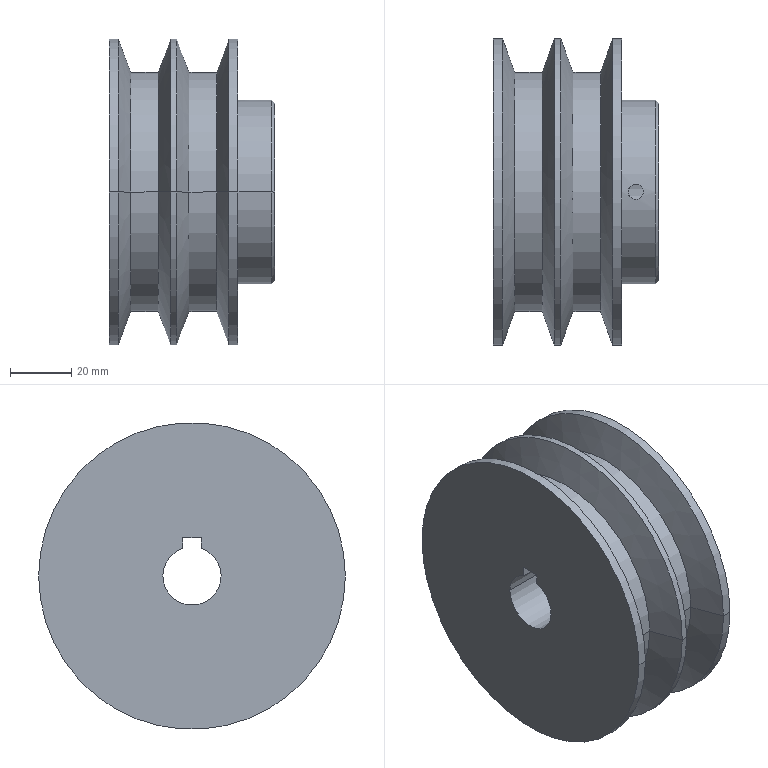Part | SolidWorks | features ICE 2, Chamfer 1, HoleWzd 1, Revolution 1 | 1 solid | 33 faces | box 54 x 100 x 100 mm | volume 266067 mm3 | cylinder 17 | cone 10 | plane 6 | commonest cylinder face diameters 100 x6 78 x4 19 x3 5 x2 60 x2
STEP:
#1=CARTESIAN_POINT('',(54.,29.,0.));
#2=VERTEX_POINT('',#1);
#3=CARTESIAN_POINT('',(54.,-29.,0.));
#4=VERTEX_POINT('',#3);
#5=CARTESIAN_POINT('',(54.,0.,0.));
#6=DIRECTION('',(1.,0.,0.));
#7=DIRECTION('',(0.,1.,0.));
#8=AXIS2_PLACEMENT_3D('',#5,#6,#7);
#9=CIRCLE('',#8,29.);
#10=EDGE_CURVE('',#2,#4,#9,.T.);
#11=ORIENTED_EDGE('',*,*,#10,.F.);
#12=CARTESIAN_POINT('',(53.,30.,0.));
#13=VERTEX_POINT('',#12);
#14=CARTESIAN_POINT('',(54.,29.,0.));
#15=DIRECTION('',(-0.7071,0.7071,0.));
#16=VECTOR('',#15,1000.);
#17=LINE('',#14,#16);
#18=EDGE_CURVE('',#2,#13,#17,.T.);
#19=ORIENTED_EDGE('',*,*,#18,.T.);
#20=CARTESIAN_POINT('',(53.,-30.,0.));
#21=VERTEX_POINT('',#20);
#22=CARTESIAN_POINT('',(53.,0.,0.));
#23=DIRECTION('',(-1.,0.,0.));
#24=DIRECTION('',(0.,1.,0.));
#25=AXIS2_PLACEMENT_3D('',#22,#23,#24);
#26=CIRCLE('',#25,30.);
#27=EDGE_CURVE('',#21,#13,#26,.T.);
#28=ORIENTED_EDGE('',*,*,#27,.F.);
#29=CARTESIAN_POINT('',(54.,-29.,0.));
#30=DIRECTION('',(-0.7071,-0.7071,0.));
#31=VECTOR('',#30,1000.);
#32=LINE('',#29,#31);
#33=EDGE_CURVE('',#4,#21,#32,.T.);
#34=ORIENTED_EDGE('',*,*,#33,.F.);
#35=EDGE_LOOP('',(#11,#19,#28,#34));
#36=FACE_OUTER_BOUND('',#35,.T.);
#37=CARTESIAN_POINT('',(54.,0.,0.));
#38=DIRECTION('',(-1.,0.,0.));
#39=DIRECTION('',(0.,-1.,0.));
#40=AXIS2_PLACEMENT_3D('',#37,#38,#39);
#41=CONICAL_SURFACE('',#40,29.,0.7854);
#42=ADVANCED_FACE('',(#36),#41,.T.);
#43=CARTESIAN_POINT('',(44.,0.,30.));
#44=VERTEX_POINT('',#43);
#45=CARTESIAN_POINT('',(49.,0.,30.));
#46=VERTEX_POINT('',#45);
#47=CARTESIAN_POINT('',(44.,0.,30.));
#48=CARTESIAN_POINT('',(44.,-0.1653,30.));
#49=CARTESIAN_POINT('',(44.016,-0.3277,29.999));
#50=CARTESIAN_POINT('',(44.08,-0.6474,29.993));
#51=CARTESIAN_POINT('',(44.128,-0.8062,29.99));
#52=CARTESIAN_POINT('',(44.253,-1.109,29.98));
#53=CARTESIAN_POINT('',(44.33,-1.253,29.974));
#54=CARTESIAN_POINT('',(44.512,-1.524,29.962));
#55=CARTESIAN_POINT('',(44.617,-1.653,29.955));
#56=CARTESIAN_POINT('',(44.848,-1.883,29.941));
#57=CARTESIAN_POINT('',(44.974,-1.987,29.934));
#58=CARTESIAN_POINT('',(45.247,-2.17,29.922));
#59=CARTESIAN_POINT('',(45.392,-2.247,29.916));
#60=CARTESIAN_POINT('',(45.693,-2.372,29.906));
#61=CARTESIAN_POINT('',(45.851,-2.42,29.902));
#62=CARTESIAN_POINT('',(46.174,-2.484,29.897));
#63=CARTESIAN_POINT('',(46.336,-2.5,29.896));
#64=CARTESIAN_POINT('',(46.662,-2.5,29.896));
#65=CARTESIAN_POINT('',(46.828,-2.484,29.897));
#66=CARTESIAN_POINT('',(47.149,-2.42,29.902));
#67=CARTESIAN_POINT('',(47.305,-2.373,29.906));
#68=CARTESIAN_POINT('',(47.607,-2.247,29.916));
#69=CARTESIAN_POINT('',(47.754,-2.169,29.922));
#70=CARTESIAN_POINT('',(48.024,-1.988,29.934));
#71=CARTESIAN_POINT('',(48.151,-1.885,29.941));
#72=CARTESIAN_POINT('',(48.384,-1.651,29.955));
#73=CARTESIAN_POINT('',(48.488,-1.525,29.962));
#74=CARTESIAN_POINT('',(48.669,-1.254,29.974));
#75=CARTESIAN_POINT('',(48.747,-1.108,29.98));
#76=CARTESIAN_POINT('',(48.872,-0.8053,29.99));
#77=CARTESIAN_POINT('',(48.92,-0.6495,29.993));
#78=CARTESIAN_POINT('',(48.984,-0.329,29.999));
#79=CARTESIAN_POINT('',(49.,-0.1632,30.));
#80=CARTESIAN_POINT('',(49.,0.,30.));
#81=B_SPLINE_CURVE_WITH_KNOTS('',3,(#47,#48,#49,#50,#51,#52,#53,#54,#55,#56,#57,#58,#59,#60,#61,#62,#63,#64,#65,#66,#67,#68,#69,#70,#71,#72,#73,#74,#75,#76,#77,#78,#79,#80),.UNSPECIFIED.,.F.,.F.,(4,2,2,2,2,2,2,2,2,2,2,2,2,2,2,2,4),(0.,0.0004887,0.0009774,0.001466,0.001955,0.002444,0.002932,0.003421,0.00391,0.004398,0.004887,0.005376,0.005865,0.006353,0.006842,0.007331,0.00782),.UNSPECIFIED.);
#82=EDGE_CURVE('',#44,#46,#81,.T.);
#83=ORIENTED_EDGE('',*,*,#82,.T.);
#84=CARTESIAN_POINT('',(49.,0.,12.5));
#85=VERTEX_POINT('',#84);
#86=CARTESIAN_POINT('',(49.,0.,0.));
#87=DIRECTION('',(0.,0.,-1.));
#88=VECTOR('',#87,1000.);
#89=LINE('',#86,#88);
#90=EDGE_CURVE('',#46,#85,#89,.T.);
#91=ORIENTED_EDGE('',*,*,#90,.T.);
#92=CARTESIAN_POINT('',(44.,0.,12.5));
#93=VERTEX_POINT('',#92);
#94=CARTESIAN_POINT('',(46.5,0.,12.5));
#95=DIRECTION('',(0.,0.,-1.));
#96=DIRECTION('',(1.,0.,0.));
#97=AXIS2_PLACEMENT_3D('',#94,#95,#96);
#98=CIRCLE('',#97,2.5);
#99=EDGE_CURVE('',#85,#93,#98,.T.);
#100=ORIENTED_EDGE('',*,*,#99,.T.);
#101=CARTESIAN_POINT('',(44.,0.,0.));
#102=DIRECTION('',(0.,0.,-1.));
#103=VECTOR('',#102,1000.);
#104=LINE('',#101,#103);
#105=EDGE_CURVE('',#44,#93,#104,.T.);
#106=ORIENTED_EDGE('',*,*,#105,.F.);
#107=EDGE_LOOP('',(#83,#91,#100,#106));
#108=FACE_OUTER_BOUND('',#107,.T.);
#109=CARTESIAN_POINT('',(46.5,0.,0.));
#110=DIRECTION('',(0.,0.,-1.));
#111=DIRECTION('',(-1.,0.,0.));
#112=AXIS2_PLACEMENT_3D('',#109,#110,#111);
#113=CYLINDRICAL_SURFACE('',#112,2.5);
#114=ADVANCED_FACE('',(#108),#113,.F.);
#115=CARTESIAN_POINT('',(0.,9.5,0.));
#116=VERTEX_POINT('',#115);
#117=CARTESIAN_POINT('',(0.,-9.5,0.));
#118=VERTEX_POINT('',#117);
#119=CARTESIAN_POINT('',(0.,0.,0.));
#120=DIRECTION('',(-1.,0.,0.));
#121=DIRECTION('',(0.,-1.,0.));
#122=AXIS2_PLACEMENT_3D('',#119,#120,#121);
#123=CIRCLE('',#122,9.5);
#124=EDGE_CURVE('',#116,#118,#123,.T.);
#125=ORIENTED_EDGE('',*,*,#124,.T.);
#126=CARTESIAN_POINT('',(54.,-9.5,0.));
#127=VERTEX_POINT('',#126);
#128=CARTESIAN_POINT('',(-16.,-9.5,0.));
#129=DIRECTION('',(1.,0.,0.));
#130=VECTOR('',#129,1000.);
#131=LINE('',#128,#130);
#132=EDGE_CURVE('',#118,#127,#131,.T.);
#133=ORIENTED_EDGE('',*,*,#132,.T.);
#134=CARTESIAN_POINT('',(54.,9.5,0.));
#135=VERTEX_POINT('',#134);
#136=CARTESIAN_POINT('',(54.,0.,0.));
#137=DIRECTION('',(1.,0.,0.));
#138=DIRECTION('',(0.,1.,0.));
#139=AXIS2_PLACEMENT_3D('',#136,#137,#138);
#140=CIRCLE('',#139,9.5);
#141=EDGE_CURVE('',#127,#135,#140,.T.);
#142=ORIENTED_EDGE('',*,*,#141,.T.);
#143=CARTESIAN_POINT('',(-16.,9.5,0.));
#144=DIRECTION('',(1.,0.,0.));
#145=VECTOR('',#144,1000.);
#146=LINE('',#143,#145);
#147=EDGE_CURVE('',#116,#135,#146,.T.);
#148=ORIENTED_EDGE('',*,*,#147,.F.);
#149=EDGE_LOOP('',(#125,#133,#142,#148));
#150=FACE_OUTER_BOUND('',#149,.T.);
#151=CARTESIAN_POINT('',(-16.,0.,0.));
#152=DIRECTION('',(1.,0.,0.));
#153=DIRECTION('',(0.,1.,0.));
#154=AXIS2_PLACEMENT_3D('',#151,#152,#153);
#155=CYLINDRICAL_SURFACE('',#154,9.5);
#156=ADVANCED_FACE('',(#150),#155,.F.);
#157=CARTESIAN_POINT('',(0.,3.,9.014));
#158=VERTEX_POINT('',#157);
#159=CARTESIAN_POINT('',(0.,0.,0.));
#160=DIRECTION('',(-1.,0.,0.));
#161=DIRECTION('',(0.,-1.,0.));
#162=AXIS2_PLACEMENT_3D('',#159,#160,#161);
#163=CIRCLE('',#162,9.5);
#164=EDGE_CURVE('',#158,#116,#163,.T.);
#165=ORIENTED_EDGE('',*,*,#164,.T.);
#166=ORIENTED_EDGE('',*,*,#147,.T.);
#167=CARTESIAN_POINT('',(54.,3.,9.014));
#168=VERTEX_POINT('',#167);
#169=CARTESIAN_POINT('',(54.,0.,0.));
#170=DIRECTION('',(1.,0.,0.));
#171=DIRECTION('',(0.,1.,0.));
#172=AXIS2_PLACEMENT_3D('',#169,#170,#171);
#173=CIRCLE('',#172,9.5);
#174=EDGE_CURVE('',#135,#168,#173,.T.);
#175=ORIENTED_EDGE('',*,*,#174,.T.);
#176=CARTESIAN_POINT('',(-16.,3.,9.014));
#177=DIRECTION('',(-1.,0.,0.));
#178=VECTOR('',#177,1000.);
#179=LINE('',#176,#178);
#180=EDGE_CURVE('',#168,#158,#179,.T.);
#181=ORIENTED_EDGE('',*,*,#180,.T.);
#182=EDGE_LOOP('',(#165,#166,#175,#181));
#183=FACE_OUTER_BOUND('',#182,.T.);
#184=CARTESIAN_POINT('',(-16.,0.,0.));
#185=DIRECTION('',(1.,0.,0.));
#186=DIRECTION('',(0.,1.,0.));
#187=AXIS2_PLACEMENT_3D('',#184,#185,#186);
#188=CYLINDRICAL_SURFACE('',#187,9.5);
#189=ADVANCED_FACE('',(#183),#188,.F.);
#190=ORIENTED_EDGE('',*,*,#82,.F.);
#191=CARTESIAN_POINT('',(49.,0.,30.));
#192=CARTESIAN_POINT('',(49.,0.1632,30.));
#193=CARTESIAN_POINT('',(48.984,0.3254,29.999));
#194=CARTESIAN_POINT('',(48.92,0.6478,29.993));
#195=CARTESIAN_POINT('',(48.872,0.8057,29.99));
#196=CARTESIAN_POINT('',(48.748,1.107,29.98));
#197=CARTESIAN_POINT('',(48.67,1.252,29.974));
#198=CARTESIAN_POINT('',(48.488,1.525,29.962));
#199=CARTESIAN_POINT('',(48.384,1.651,29.955));
#200=CARTESIAN_POINT('',(48.154,1.882,29.941));
#201=CARTESIAN_POINT('',(48.025,1.987,29.934));
#202=CARTESIAN_POINT('',(47.754,2.169,29.922));
#203=CARTESIAN_POINT('',(47.61,2.246,29.916));
#204=CARTESIAN_POINT('',(47.308,2.372,29.906));
#205=CARTESIAN_POINT('',(47.149,2.42,29.902));
#206=CARTESIAN_POINT('',(46.829,2.484,29.897));
#207=CARTESIAN_POINT('',(46.667,2.5,29.896));
#208=CARTESIAN_POINT('',(46.337,2.5,29.896));
#209=CARTESIAN_POINT('',(46.174,2.484,29.897));
#210=CARTESIAN_POINT('',(45.854,2.421,29.902));
#211=CARTESIAN_POINT('',(45.696,2.373,29.906));
#212=CARTESIAN_POINT('',(45.393,2.247,29.916));
#213=CARTESIAN_POINT('',(45.249,2.171,29.921));
#214=CARTESIAN_POINT('',(44.978,1.99,29.934));
#215=CARTESIAN_POINT('',(44.849,1.884,29.941));
#216=CARTESIAN_POINT('',(44.618,1.654,29.955));
#217=CARTESIAN_POINT('',(44.515,1.528,29.961));
#218=CARTESIAN_POINT('',(44.332,1.255,29.974));
#219=CARTESIAN_POINT('',(44.254,1.11,29.98));
#220=CARTESIAN_POINT('',(44.066,0.6587,29.994));
#221=CARTESIAN_POINT('',(44.,0.3304,30.));
#222=CARTESIAN_POINT('',(44.,0.,30.));
#223=B_SPLINE_CURVE_WITH_KNOTS('',3,(#191,#192,#193,#194,#195,#196,#197,#198,#199,#200,#201,#202,#203,#204,#205,#206,#207,#208,#209,#210,#211,#212,#213,#214,#215,#216,#217,#218,#219,#220,#221,#222),.UNSPECIFIED.,.F.,.F.,(4,2,2,2,2,2,2,2,2,2,2,2,2,2,2,4),(0.00782,0.008308,0.008797,0.009285,0.009774,0.01026,0.01075,0.01124,0.01173,0.01222,0.01271,0.01319,0.01368,0.01417,0.01466,0.01564),.UNSPECIFIED.);
#224=EDGE_CURVE('',#46,#44,#223,.T.);
#225=ORIENTED_EDGE('',*,*,#224,.F.);
#226=EDGE_LOOP('',(#190,#225));
#227=FACE_BOUND('',#226,.T.);
#228=CARTESIAN_POINT('',(42.,30.,0.));
#229=VERTEX_POINT('',#228);
#230=CARTESIAN_POINT('',(42.,-30.,0.));
#231=VERTEX_POINT('',#230);
#232=CARTESIAN_POINT('',(42.,0.,0.));
#233=DIRECTION('',(1.,0.,0.));
#234=DIRECTION('',(0.,1.,0.));
#235=AXIS2_PLACEMENT_3D('',#232,#233,#234);
#236=CIRCLE('',#235,30.);
#237=EDGE_CURVE('',#229,#231,#236,.T.);
#238=ORIENTED_EDGE('',*,*,#237,.T.);
#239=CARTESIAN_POINT('',(54.,-30.,0.));
#240=DIRECTION('',(1.,0.,0.));
#241=VECTOR('',#240,1000.);
#242=LINE('',#239,#241);
#243=EDGE_CURVE('',#231,#21,#242,.T.);
#244=ORIENTED_EDGE('',*,*,#243,.T.);
#245=ORIENTED_EDGE('',*,*,#27,.T.);
#246=CARTESIAN_POINT('',(54.,30.,0.));
#247=DIRECTION('',(1.,0.,0.));
#248=VECTOR('',#247,1000.);
#249=LINE('',#246,#248);
#250=EDGE_CURVE('',#229,#13,#249,.T.);
#251=ORIENTED_EDGE('',*,*,#250,.F.);
#252=EDGE_LOOP('',(#238,#244,#245,#251));
#253=FACE_OUTER_BOUND('',#252,.T.);
#254=CARTESIAN_POINT('',(54.,0.,0.));
#255=DIRECTION('',(1.,0.,0.));
#256=DIRECTION('',(0.,1.,0.));
#257=AXIS2_PLACEMENT_3D('',#254,#255,#256);
#258=CYLINDRICAL_SURFACE('',#257,30.);
#259=ADVANCED_FACE('',(#227,#253),#258,.T.);
#260=CARTESIAN_POINT('',(39.,50.,0.));
#261=VERTEX_POINT('',#260);
#262=CARTESIAN_POINT('',(39.,-50.,0.));
#263=VERTEX_POINT('',#262);
#264=CARTESIAN_POINT('',(39.,0.,0.));
#265=DIRECTION('',(1.,0.,0.));
#266=DIRECTION('',(0.,1.,0.));
#267=AXIS2_PLACEMENT_3D('',#264,#265,#266);
#268=CIRCLE('',#267,50.);
#269=EDGE_CURVE('',#261,#263,#268,.T.);
#270=ORIENTED_EDGE('',*,*,#269,.T.);
#271=CARTESIAN_POINT('',(42.,-50.,0.));
#272=VERTEX_POINT('',#271);
#273=CARTESIAN_POINT('',(54.,-50.,0.));
#274=DIRECTION('',(1.,0.,0.));
#275=VECTOR('',#274,1000.);
#276=LINE('',#273,#275);
#277=EDGE_CURVE('',#263,#272,#276,.T.);
#278=ORIENTED_EDGE('',*,*,#277,.T.);
#279=CARTESIAN_POINT('',(42.,50.,0.));
#280=VERTEX_POINT('',#279);
#281=CARTESIAN_POINT('',(42.,0.,0.));
#282=DIRECTION('',(1.,0.,0.));
#283=DIRECTION('',(0.,1.,0.));
#284=AXIS2_PLACEMENT_3D('',#281,#282,#283);
#285=CIRCLE('',#284,50.);
#286=EDGE_CURVE('',#280,#272,#285,.T.);
#287=ORIENTED_EDGE('',*,*,#286,.F.);
#288=CARTESIAN_POINT('',(54.,50.,0.));
#289=DIRECTION('',(1.,0.,0.));
#290=VECTOR('',#289,1000.);
#291=LINE('',#288,#290);
#292=EDGE_CURVE('',#261,#280,#291,.T.);
#293=ORIENTED_EDGE('',*,*,#292,.F.);
#294=EDGE_LOOP('',(#270,#278,#287,#293));
#295=FACE_OUTER_BOUND('',#294,.T.);
#296=CARTESIAN_POINT('',(54.,0.,0.));
#297=DIRECTION('',(1.,0.,0.));
#298=DIRECTION('',(0.,1.,0.));
#299=AXIS2_PLACEMENT_3D('',#296,#297,#298);
#300=CYLINDRICAL_SURFACE('',#299,50.);
#301=ADVANCED_FACE('',(#295),#300,.T.);
#302=CARTESIAN_POINT('',(34.996,39.,0.));
#303=VERTEX_POINT('',#302);
#304=CARTESIAN_POINT('',(34.996,-39.,0.));
#305=VERTEX_POINT('',#304);
#306=CARTESIAN_POINT('',(34.996,0.,0.));
#307=DIRECTION('',(1.,0.,0.));
#308=DIRECTION('',(0.,1.,0.));
#309=AXIS2_PLACEMENT_3D('',#306,#307,#308);
#310=CIRCLE('',#309,39.);
#311=EDGE_CURVE('',#303,#305,#310,.T.);
#312=ORIENTED_EDGE('',*,*,#311,.T.);
#313=CARTESIAN_POINT('',(39.,-50.,0.));
#314=DIRECTION('',(0.342,-0.9397,0.));
#315=VECTOR('',#314,1000.);
#316=LINE('',#313,#315);
#317=EDGE_CURVE('',#305,#263,#316,.T.);
#318=ORIENTED_EDGE('',*,*,#317,.T.);
#319=ORIENTED_EDGE('',*,*,#269,.F.);
#320=CARTESIAN_POINT('',(39.,50.,0.));
#321=DIRECTION('',(0.342,0.9397,0.));
#322=VECTOR('',#321,1000.);
#323=LINE('',#320,#322);
#324=EDGE_CURVE('',#303,#261,#323,.T.);
#325=ORIENTED_EDGE('',*,*,#324,.F.);
#326=EDGE_LOOP('',(#312,#318,#319,#325));
#327=FACE_OUTER_BOUND('',#326,.T.);
#328=CARTESIAN_POINT('',(39.,0.,0.));
#329=DIRECTION('',(1.,0.,0.));
#330=DIRECTION('',(0.,1.,0.));
#331=AXIS2_PLACEMENT_3D('',#328,#329,#330);
#332=CONICAL_SURFACE('',#331,50.,1.222);
#333=ADVANCED_FACE('',(#327),#332,.T.);
#334=CARTESIAN_POINT('',(26.004,39.,0.));
#335=VERTEX_POINT('',#334);
#336=CARTESIAN_POINT('',(26.004,-39.,0.));
#337=VERTEX_POINT('',#336);
#338=CARTESIAN_POINT('',(26.004,0.,0.));
#339=DIRECTION('',(1.,0.,0.));
#340=DIRECTION('',(0.,1.,0.));
#341=AXIS2_PLACEMENT_3D('',#338,#339,#340);
#342=CIRCLE('',#341,39.);
#343=EDGE_CURVE('',#335,#337,#342,.T.);
#344=ORIENTED_EDGE('',*,*,#343,.T.);
#345=CARTESIAN_POINT('',(54.,-39.,0.));
#346=DIRECTION('',(1.,0.,0.));
#347=VECTOR('',#346,1000.);
#348=LINE('',#345,#347);
#349=EDGE_CURVE('',#337,#305,#348,.T.);
#350=ORIENTED_EDGE('',*,*,#349,.T.);
#351=ORIENTED_EDGE('',*,*,#311,.F.);
#352=CARTESIAN_POINT('',(54.,39.,0.));
#353=DIRECTION('',(1.,0.,0.));
#354=VECTOR('',#353,1000.);
#355=LINE('',#352,#354);
#356=EDGE_CURVE('',#335,#303,#355,.T.);
#357=ORIENTED_EDGE('',*,*,#356,.F.);
#358=EDGE_LOOP('',(#344,#350,#351,#357));
#359=FACE_OUTER_BOUND('',#358,.T.);
#360=CARTESIAN_POINT('',(54.,0.,0.));
#361=DIRECTION('',(1.,0.,0.));
#362=DIRECTION('',(0.,1.,0.));
#363=AXIS2_PLACEMENT_3D('',#360,#361,#362);
#364=CYLINDRICAL_SURFACE('',#363,39.);
#365=ADVANCED_FACE('',(#359),#364,.T.);
#366=ORIENTED_EDGE('',*,*,#343,.F.);
#367=CARTESIAN_POINT('',(22.,50.,0.));
#368=VERTEX_POINT('',#367);
#369=CARTESIAN_POINT('',(26.004,39.,0.));
#370=DIRECTION('',(-0.342,0.9397,0.));
#371=VECTOR('',#370,1000.);
#372=LINE('',#369,#371);
#373=EDGE_CURVE('',#335,#368,#372,.T.);
#374=ORIENTED_EDGE('',*,*,#373,.T.);
#375=CARTESIAN_POINT('',(22.,-50.,0.));
#376=VERTEX_POINT('',#375);
#377=CARTESIAN_POINT('',(22.,0.,0.));
#378=DIRECTION('',(1.,0.,0.));
#379=DIRECTION('',(0.,1.,0.));
#380=AXIS2_PLACEMENT_3D('',#377,#378,#379);
#381=CIRCLE('',#380,50.);
#382=EDGE_CURVE('',#368,#376,#381,.T.);
#383=ORIENTED_EDGE('',*,*,#382,.T.);
#384=CARTESIAN_POINT('',(26.004,-39.,0.));
#385=DIRECTION('',(-0.342,-0.9397,0.));
#386=VECTOR('',#385,1000.);
#387=LINE('',#384,#386);
#388=EDGE_CURVE('',#337,#376,#387,.T.);
#389=ORIENTED_EDGE('',*,*,#388,.F.);
#390=EDGE_LOOP('',(#366,#374,#383,#389));
#391=FACE_OUTER_BOUND('',#390,.T.);
#392=CARTESIAN_POINT('',(26.004,0.,0.));
#393=DIRECTION('',(-1.,0.,0.));
#394=DIRECTION('',(0.,-1.,0.));
#395=AXIS2_PLACEMENT_3D('',#392,#393,#394);
#396=CONICAL_SURFACE('',#395,39.,1.222);
#397=ADVANCED_FACE('',(#391),#396,.T.);
#398=CARTESIAN_POINT('',(20.,50.,0.));
#399=VERTEX_POINT('',#398);
#400=CARTESIAN_POINT('',(20.,-50.,0.));
#401=VERTEX_POINT('',#400);
#402=CARTESIAN_POINT('',(20.,0.,0.));
#403=DIRECTION('',(1.,0.,0.));
#404=DIRECTION('',(0.,1.,0.));
#405=AXIS2_PLACEMENT_3D('',#402,#403,#404);
#406=CIRCLE('',#405,50.);
#407=EDGE_CURVE('',#399,#401,#406,.T.);
#408=ORIENTED_EDGE('',*,*,#407,.T.);
#409=CARTESIAN_POINT('',(54.,-50.,0.));
#410=DIRECTION('',(1.,0.,0.));
#411=VECTOR('',#410,1000.);
#412=LINE('',#409,#411);
#413=EDGE_CURVE('',#401,#376,#412,.T.);
#414=ORIENTED_EDGE('',*,*,#413,.T.);
#415=ORIENTED_EDGE('',*,*,#382,.F.);
#416=CARTESIAN_POINT('',(54.,50.,0.));
#417=DIRECTION('',(1.,0.,0.));
#418=VECTOR('',#417,1000.);
#419=LINE('',#416,#418);
#420=EDGE_CURVE('',#399,#368,#419,.T.);
#421=ORIENTED_EDGE('',*,*,#420,.F.);
#422=EDGE_LOOP('',(#408,#414,#415,#421));
#423=FACE_OUTER_BOUND('',#422,.T.);
#424=CARTESIAN_POINT('',(54.,0.,0.));
#425=DIRECTION('',(1.,0.,0.));
#426=DIRECTION('',(0.,1.,0.));
#427=AXIS2_PLACEMENT_3D('',#424,#425,#426);
#428=CYLINDRICAL_SURFACE('',#427,50.);
#429=ADVANCED_FACE('',(#423),#428,.T.);
#430=CARTESIAN_POINT('',(15.996,39.,0.));
#431=VERTEX_POINT('',#430);
#432=CARTESIAN_POINT('',(15.996,-39.,0.));
#433=VERTEX_POINT('',#432);
#434=CARTESIAN_POINT('',(15.996,0.,0.));
#435=DIRECTION('',(1.,0.,0.));
#436=DIRECTION('',(0.,1.,0.));
#437=AXIS2_PLACEMENT_3D('',#434,#435,#436);
#438=CIRCLE('',#437,39.);
#439=EDGE_CURVE('',#431,#433,#438,.T.);
#440=ORIENTED_EDGE('',*,*,#439,.T.);
#441=CARTESIAN_POINT('',(20.,-50.,0.));
#442=DIRECTION('',(0.342,-0.9397,0.));
#443=VECTOR('',#442,1000.);
#444=LINE('',#441,#443);
#445=EDGE_CURVE('',#433,#401,#444,.T.);
#446=ORIENTED_EDGE('',*,*,#445,.T.);
#447=ORIENTED_EDGE('',*,*,#407,.F.);
#448=CARTESIAN_POINT('',(20.,50.,0.));
#449=DIRECTION('',(0.342,0.9397,0.));
#450=VECTOR('',#449,1000.);
#451=LINE('',#448,#450);
#452=EDGE_CURVE('',#431,#399,#451,.T.);
#453=ORIENTED_EDGE('',*,*,#452,.F.);
#454=EDGE_LOOP('',(#440,#446,#447,#453));
#455=FACE_OUTER_BOUND('',#454,.T.);
#456=CARTESIAN_POINT('',(20.,0.,0.));
#457=DIRECTION('',(1.,0.,0.));
#458=DIRECTION('',(0.,1.,0.));
#459=AXIS2_PLACEMENT_3D('',#456,#457,#458);
#460=CONICAL_SURFACE('',#459,50.,1.222);
#461=ADVANCED_FACE('',(#455),#460,.T.);
#462=CARTESIAN_POINT('',(7.004,39.,0.));
#463=VERTEX_POINT('',#462);
#464=CARTESIAN_POINT('',(7.004,-39.,0.));
#465=VERTEX_POINT('',#464);
#466=CARTESIAN_POINT('',(7.004,0.,0.));
#467=DIRECTION('',(1.,0.,0.));
#468=DIRECTION('',(0.,1.,0.));
#469=AXIS2_PLACEMENT_3D('',#466,#467,#468);
#470=CIRCLE('',#469,39.);
#471=EDGE_CURVE('',#463,#465,#470,.T.);
#472=ORIENTED_EDGE('',*,*,#471,.T.);
#473=CARTESIAN_POINT('',(54.,-39.,0.));
#474=DIRECTION('',(1.,0.,0.));
#475=VECTOR('',#474,1000.);
#476=LINE('',#473,#475);
#477=EDGE_CURVE('',#465,#433,#476,.T.);
#478=ORIENTED_EDGE('',*,*,#477,.T.);
#479=ORIENTED_EDGE('',*,*,#439,.F.);
#480=CARTESIAN_POINT('',(54.,39.,0.));
#481=DIRECTION('',(1.,0.,0.));
#482=VECTOR('',#481,1000.);
#483=LINE('',#480,#482);
#484=EDGE_CURVE('',#463,#431,#483,.T.);
#485=ORIENTED_EDGE('',*,*,#484,.F.);
#486=EDGE_LOOP('',(#472,#478,#479,#485));
#487=FACE_OUTER_BOUND('',#486,.T.);
#488=CARTESIAN_POINT('',(54.,0.,0.));
#489=DIRECTION('',(1.,0.,0.));
#490=DIRECTION('',(0.,1.,0.));
#491=AXIS2_PLACEMENT_3D('',#488,#489,#490);
#492=CYLINDRICAL_SURFACE('',#491,39.);
#493=ADVANCED_FACE('',(#487),#492,.T.);
#494=ORIENTED_EDGE('',*,*,#471,.F.);
#495=CARTESIAN_POINT('',(3.,50.,0.));
#496=VERTEX_POINT('',#495);
#497=CARTESIAN_POINT('',(7.004,39.,0.));
#498=DIRECTION('',(-0.342,0.9397,0.));
#499=VECTOR('',#498,1000.);
#500=LINE('',#497,#499);
#501=EDGE_CURVE('',#463,#496,#500,.T.);
#502=ORIENTED_EDGE('',*,*,#501,.T.);
#503=CARTESIAN_POINT('',(3.,-50.,0.));
#504=VERTEX_POINT('',#503);
#505=CARTESIAN_POINT('',(3.,0.,0.));
#506=DIRECTION('',(1.,0.,0.));
#507=DIRECTION('',(0.,1.,0.));
#508=AXIS2_PLACEMENT_3D('',#505,#506,#507);
#509=CIRCLE('',#508,50.);
#510=EDGE_CURVE('',#496,#504,#509,.T.);
#511=ORIENTED_EDGE('',*,*,#510,.T.);
#512=CARTESIAN_POINT('',(7.004,-39.,0.));
#513=DIRECTION('',(-0.342,-0.9397,0.));
#514=VECTOR('',#513,1000.);
#515=LINE('',#512,#514);
#516=EDGE_CURVE('',#465,#504,#515,.T.);
#517=ORIENTED_EDGE('',*,*,#516,.F.);
#518=EDGE_LOOP('',(#494,#502,#511,#517));
#519=FACE_OUTER_BOUND('',#518,.T.);
#520=CARTESIAN_POINT('',(7.004,0.,0.));
#521=DIRECTION('',(-1.,0.,0.));
#522=DIRECTION('',(0.,-1.,0.));
#523=AXIS2_PLACEMENT_3D('',#520,#521,#522);
#524=CONICAL_SURFACE('',#523,39.,1.222);
#525=ADVANCED_FACE('',(#519),#524,.T.);
#526=CARTESIAN_POINT('',(0.,50.,0.));
#527=VERTEX_POINT('',#526);
#528=CARTESIAN_POINT('',(0.,-50.,0.));
#529=VERTEX_POINT('',#528);
#530=CARTESIAN_POINT('',(0.,0.,0.));
#531=DIRECTION('',(1.,0.,0.));
#532=DIRECTION('',(0.,1.,0.));
#533=AXIS2_PLACEMENT_3D('',#530,#531,#532);
#534=CIRCLE('',#533,50.);
#535=EDGE_CURVE('',#527,#529,#534,.T.);
#536=ORIENTED_EDGE('',*,*,#535,.T.);
#537=CARTESIAN_POINT('',(54.,-50.,0.));
#538=DIRECTION('',(1.,0.,0.));
#539=VECTOR('',#538,1000.);
#540=LINE('',#537,#539);
#541=EDGE_CURVE('',#529,#504,#540,.T.);
#542=ORIENTED_EDGE('',*,*,#541,.T.);
#543=ORIENTED_EDGE('',*,*,#510,.F.);
#544=CARTESIAN_POINT('',(54.,50.,0.));
#545=DIRECTION('',(1.,0.,0.));
#546=VECTOR('',#545,1000.);
#547=LINE('',#544,#546);
#548=EDGE_CURVE('',#527,#496,#547,.T.);
#549=ORIENTED_EDGE('',*,*,#548,.F.);
#550=EDGE_LOOP('',(#536,#542,#543,#549));
#551=FACE_OUTER_BOUND('',#550,.T.);
#552=CARTESIAN_POINT('',(54.,0.,0.));
#553=DIRECTION('',(1.,0.,0.));
#554=DIRECTION('',(0.,1.,0.));
#555=AXIS2_PLACEMENT_3D('',#552,#553,#554);
#556=CYLINDRICAL_SURFACE('',#555,50.);
#557=ADVANCED_FACE('',(#551),#556,.T.);
#558=CARTESIAN_POINT('',(0.,-3.,9.014));
#559=VERTEX_POINT('',#558);
#560=CARTESIAN_POINT('',(0.,-3.,12.5));
#561=VERTEX_POINT('',#560);
#562=CARTESIAN_POINT('',(0.,-3.,0.));
#563=DIRECTION('',(0.,0.,1.));
#564=VECTOR('',#563,1000.);
#565=LINE('',#562,#564);
#566=EDGE_CURVE('',#559,#561,#565,.T.);
#567=ORIENTED_EDGE('',*,*,#566,.F.);
#568=CARTESIAN_POINT('',(0.,0.,0.));
#569=DIRECTION('',(-1.,0.,0.));
#570=DIRECTION('',(0.,-1.,0.));
#571=AXIS2_PLACEMENT_3D('',#568,#569,#570);
#572=CIRCLE('',#571,9.5);
#573=EDGE_CURVE('',#118,#559,#572,.T.);
#574=ORIENTED_EDGE('',*,*,#573,.F.);
#575=ORIENTED_EDGE('',*,*,#124,.F.);
#576=ORIENTED_EDGE('',*,*,#164,.F.);
#577=CARTESIAN_POINT('',(0.,3.,12.5));
#578=VERTEX_POINT('',#577);
#579=CARTESIAN_POINT('',(0.,3.,0.));
#580=DIRECTION('',(0.,0.,-1.));
#581=VECTOR('',#580,1000.);
#582=LINE('',#579,#581);
#583=EDGE_CURVE('',#578,#158,#582,.T.);
#584=ORIENTED_EDGE('',*,*,#583,.F.);
#585=CARTESIAN_POINT('',(0.,0.,12.5));
#586=DIRECTION('',(0.,1.,0.));
#587=VECTOR('',#586,1000.);
#588=LINE('',#585,#587);
#589=EDGE_CURVE('',#561,#578,#588,.T.);
#590=ORIENTED_EDGE('',*,*,#589,.F.);
#591=EDGE_LOOP('',(#567,#574,#575,#576,#584,#590));
#592=FACE_BOUND('',#591,.T.);
#593=ORIENTED_EDGE('',*,*,#535,.F.);
#594=CARTESIAN_POINT('',(0.,0.,0.));
#595=DIRECTION('',(1.,0.,0.));
#596=DIRECTION('',(0.,1.,0.));
#597=AXIS2_PLACEMENT_3D('',#594,#595,#596);
#598=CIRCLE('',#597,50.);
#599=EDGE_CURVE('',#529,#527,#598,.T.);
#600=ORIENTED_EDGE('',*,*,#599,.F.);
#601=EDGE_LOOP('',(#593,#600));
#602=FACE_OUTER_BOUND('',#601,.T.);
#603=CARTESIAN_POINT('',(0.,0.,0.));
#604=DIRECTION('',(-1.,0.,0.));
#605=DIRECTION('',(0.,-1.,0.));
#606=AXIS2_PLACEMENT_3D('',#603,#604,#605);
#607=PLANE('',#606);
#608=ADVANCED_FACE('',(#592,#602),#607,.T.);
#609=ORIENTED_EDGE('',*,*,#541,.F.);
#610=ORIENTED_EDGE('',*,*,#599,.T.);
#611=ORIENTED_EDGE('',*,*,#548,.T.);
#612=CARTESIAN_POINT('',(3.,0.,0.));
#613=DIRECTION('',(1.,0.,0.));
#614=DIRECTION('',(0.,1.,0.));
#615=AXIS2_PLACEMENT_3D('',#612,#613,#614);
#616=CIRCLE('',#615,50.);
#617=EDGE_CURVE('',#504,#496,#616,.T.);
#618=ORIENTED_EDGE('',*,*,#617,.F.);
#619=EDGE_LOOP('',(#609,#610,#611,#618));
#620=FACE_OUTER_BOUND('',#619,.T.);
#621=CARTESIAN_POINT('',(54.,0.,0.));
#622=DIRECTION('',(1.,0.,0.));
#623=DIRECTION('',(0.,1.,0.));
#624=AXIS2_PLACEMENT_3D('',#621,#622,#623);
#625=CYLINDRICAL_SURFACE('',#624,50.);
#626=ADVANCED_FACE('',(#620),#625,.T.);
#627=ORIENTED_EDGE('',*,*,#501,.F.);
#628=CARTESIAN_POINT('',(7.004,0.,0.));
#629=DIRECTION('',(1.,0.,0.));
#630=DIRECTION('',(0.,1.,0.));
#631=AXIS2_PLACEMENT_3D('',#628,#629,#630);
#632=CIRCLE('',#631,39.);
#633=EDGE_CURVE('',#465,#463,#632,.T.);
#634=ORIENTED_EDGE('',*,*,#633,.F.);
#635=ORIENTED_EDGE('',*,*,#516,.T.);
#636=ORIENTED_EDGE('',*,*,#617,.T.);
#637=EDGE_LOOP('',(#627,#634,#635,#636));
#638=FACE_OUTER_BOUND('',#637,.T.);
#639=CARTESIAN_POINT('',(7.004,0.,0.));
#640=DIRECTION('',(-1.,0.,0.));
#641=DIRECTION('',(0.,-1.,0.));
#642=AXIS2_PLACEMENT_3D('',#639,#640,#641);
#643=CONICAL_SURFACE('',#642,39.,1.222);
#644=ADVANCED_FACE('',(#638),#643,.T.);
#645=ORIENTED_EDGE('',*,*,#477,.F.);
#646=ORIENTED_EDGE('',*,*,#633,.T.);
#647=ORIENTED_EDGE('',*,*,#484,.T.);
#648=CARTESIAN_POINT('',(15.996,0.,0.));
#649=DIRECTION('',(1.,0.,0.));
#650=DIRECTION('',(0.,1.,0.));
#651=AXIS2_PLACEMENT_3D('',#648,#649,#650);
#652=CIRCLE('',#651,39.);
#653=EDGE_CURVE('',#433,#431,#652,.T.);
#654=ORIENTED_EDGE('',*,*,#653,.F.);
#655=EDGE_LOOP('',(#645,#646,#647,#654));
#656=FACE_OUTER_BOUND('',#655,.T.);
#657=CARTESIAN_POINT('',(54.,0.,0.));
#658=DIRECTION('',(1.,0.,0.));
#659=DIRECTION('',(0.,1.,0.));
#660=AXIS2_PLACEMENT_3D('',#657,#658,#659);
#661=CYLINDRICAL_SURFACE('',#660,39.);
#662=ADVANCED_FACE('',(#656),#661,.T.);
#663=ORIENTED_EDGE('',*,*,#445,.F.);
#664=ORIENTED_EDGE('',*,*,#653,.T.);
#665=ORIENTED_EDGE('',*,*,#452,.T.);
#666=CARTESIAN_POINT('',(20.,0.,0.));
#667=DIRECTION('',(1.,0.,0.));
#668=DIRECTION('',(0.,1.,0.));
#669=AXIS2_PLACEMENT_3D('',#666,#667,#668);
#670=CIRCLE('',#669,50.);
#671=EDGE_CURVE('',#401,#399,#670,.T.);
#672=ORIENTED_EDGE('',*,*,#671,.F.);
#673=EDGE_LOOP('',(#663,#664,#665,#672));
#674=FACE_OUTER_BOUND('',#673,.T.);
#675=CARTESIAN_POINT('',(20.,0.,0.));
#676=DIRECTION('',(1.,0.,0.));
#677=DIRECTION('',(0.,1.,0.));
#678=AXIS2_PLACEMENT_3D('',#675,#676,#677);
#679=CONICAL_SURFACE('',#678,50.,1.222);
#680=ADVANCED_FACE('',(#674),#679,.T.);
#681=ORIENTED_EDGE('',*,*,#413,.F.);
#682=ORIENTED_EDGE('',*,*,#671,.T.);
#683=ORIENTED_EDGE('',*,*,#420,.T.);
#684=CARTESIAN_POINT('',(22.,0.,0.));
#685=DIRECTION('',(1.,0.,0.));
#686=DIRECTION('',(0.,1.,0.));
#687=AXIS2_PLACEMENT_3D('',#684,#685,#686);
#688=CIRCLE('',#687,50.);
#689=EDGE_CURVE('',#376,#368,#688,.T.);
#690=ORIENTED_EDGE('',*,*,#689,.F.);
#691=EDGE_LOOP('',(#681,#682,#683,#690));
#692=FACE_OUTER_BOUND('',#691,.T.);
#693=CARTESIAN_POINT('',(54.,0.,0.));
#694=DIRECTION('',(1.,0.,0.));
#695=DIRECTION('',(0.,1.,0.));
#696=AXIS2_PLACEMENT_3D('',#693,#694,#695);
#697=CYLINDRICAL_SURFACE('',#696,50.);
#698=ADVANCED_FACE('',(#692),#697,.T.);
#699=ORIENTED_EDGE('',*,*,#373,.F.);
#700=CARTESIAN_POINT('',(26.004,0.,0.));
#701=DIRECTION('',(1.,0.,0.));
#702=DIRECTION('',(0.,1.,0.));
#703=AXIS2_PLACEMENT_3D('',#700,#701,#702);
#704=CIRCLE('',#703,39.);
#705=EDGE_CURVE('',#337,#335,#704,.T.);
#706=ORIENTED_EDGE('',*,*,#705,.F.);
#707=ORIENTED_EDGE('',*,*,#388,.T.);
#708=ORIENTED_EDGE('',*,*,#689,.T.);
#709=EDGE_LOOP('',(#699,#706,#707,#708));
#710=FACE_OUTER_BOUND('',#709,.T.);
#711=CARTESIAN_POINT('',(26.004,0.,0.));
#712=DIRECTION('',(-1.,0.,0.));
#713=DIRECTION('',(0.,-1.,0.));
#714=AXIS2_PLACEMENT_3D('',#711,#712,#713);
#715=CONICAL_SURFACE('',#714,39.,1.222);
#716=ADVANCED_FACE('',(#710),#715,.T.);
#717=ORIENTED_EDGE('',*,*,#349,.F.);
#718=ORIENTED_EDGE('',*,*,#705,.T.);
#719=ORIENTED_EDGE('',*,*,#356,.T.);
#720=CARTESIAN_POINT('',(34.996,0.,0.));
#721=DIRECTION('',(1.,0.,0.));
#722=DIRECTION('',(0.,1.,0.));
#723=AXIS2_PLACEMENT_3D('',#720,#721,#722);
#724=CIRCLE('',#723,39.);
#725=EDGE_CURVE('',#305,#303,#724,.T.);
#726=ORIENTED_EDGE('',*,*,#725,.F.);
#727=EDGE_LOOP('',(#717,#718,#719,#726));
#728=FACE_OUTER_BOUND('',#727,.T.);
#729=CARTESIAN_POINT('',(54.,0.,0.));
#730=DIRECTION('',(1.,0.,0.));
#731=DIRECTION('',(0.,1.,0.));
#732=AXIS2_PLACEMENT_3D('',#729,#730,#731);
#733=CYLINDRICAL_SURFACE('',#732,39.);
#734=ADVANCED_FACE('',(#728),#733,.T.);
#735=ORIENTED_EDGE('',*,*,#317,.F.);
#736=ORIENTED_EDGE('',*,*,#725,.T.);
#737=ORIENTED_EDGE('',*,*,#324,.T.);
#738=CARTESIAN_POINT('',(39.,0.,0.));
#739=DIRECTION('',(1.,0.,0.));
#740=DIRECTION('',(0.,1.,0.));
#741=AXIS2_PLACEMENT_3D('',#738,#739,#740);
#742=CIRCLE('',#741,50.);
#743=EDGE_CURVE('',#263,#261,#742,.T.);
#744=ORIENTED_EDGE('',*,*,#743,.F.);
#745=EDGE_LOOP('',(#735,#736,#737,#744));
#746=FACE_OUTER_BOUND('',#745,.T.);
#747=CARTESIAN_POINT('',(39.,0.,0.));
#748=DIRECTION('',(1.,0.,0.));
#749=DIRECTION('',(0.,1.,0.));
#750=AXIS2_PLACEMENT_3D('',#747,#748,#749);
#751=CONICAL_SURFACE('',#750,50.,1.222);
#752=ADVANCED_FACE('',(#746),#751,.T.);
#753=ORIENTED_EDGE('',*,*,#277,.F.);
#754=ORIENTED_EDGE('',*,*,#743,.T.);
#755=ORIENTED_EDGE('',*,*,#292,.T.);
#756=CARTESIAN_POINT('',(42.,0.,0.));
#757=DIRECTION('',(1.,0.,0.));
#758=DIRECTION('',(0.,1.,0.));
#759=AXIS2_PLACEMENT_3D('',#756,#757,#758);
#760=CIRCLE('',#759,50.);
#761=EDGE_CURVE('',#272,#280,#760,.T.);
#762=ORIENTED_EDGE('',*,*,#761,.F.);
#763=EDGE_LOOP('',(#753,#754,#755,#762));
#764=FACE_OUTER_BOUND('',#763,.T.);
#765=CARTESIAN_POINT('',(54.,0.,0.));
#766=DIRECTION('',(1.,0.,0.));
#767=DIRECTION('',(0.,1.,0.));
#768=AXIS2_PLACEMENT_3D('',#765,#766,#767);
#769=CYLINDRICAL_SURFACE('',#768,50.);
#770=ADVANCED_FACE('',(#764),#769,.T.);
#771=ORIENTED_EDGE('',*,*,#286,.T.);
#772=ORIENTED_EDGE('',*,*,#761,.T.);
#773=EDGE_LOOP('',(#771,#772));
#774=FACE_OUTER_BOUND('',#773,.T.);
#775=ORIENTED_EDGE('',*,*,#237,.F.);
#776=CARTESIAN_POINT('',(42.,0.,0.));
#777=DIRECTION('',(1.,0.,0.));
#778=DIRECTION('',(0.,1.,0.));
#779=AXIS2_PLACEMENT_3D('',#776,#777,#778);
#780=CIRCLE('',#779,30.);
#781=EDGE_CURVE('',#231,#229,#780,.T.);
#782=ORIENTED_EDGE('',*,*,#781,.F.);
#783=EDGE_LOOP('',(#775,#782));
#784=FACE_BOUND('',#783,.T.);
#785=CARTESIAN_POINT('',(42.,50.,0.));
#786=DIRECTION('',(1.,0.,0.));
#787=DIRECTION('',(0.,1.,0.));
#788=AXIS2_PLACEMENT_3D('',#785,#786,#787);
#789=PLANE('',#788);
#790=ADVANCED_FACE('',(#774,#784),#789,.T.);
#791=ORIENTED_EDGE('',*,*,#243,.F.);
#792=ORIENTED_EDGE('',*,*,#781,.T.);
#793=ORIENTED_EDGE('',*,*,#250,.T.);
#794=CARTESIAN_POINT('',(53.,0.,0.));
#795=DIRECTION('',(-1.,0.,0.));
#796=DIRECTION('',(0.,1.,0.));
#797=AXIS2_PLACEMENT_3D('',#794,#795,#796);
#798=CIRCLE('',#797,30.);
#799=EDGE_CURVE('',#13,#21,#798,.T.);
#800=ORIENTED_EDGE('',*,*,#799,.T.);
#801=EDGE_LOOP('',(#791,#792,#793,#800));
#802=FACE_OUTER_BOUND('',#801,.T.);
#803=CARTESIAN_POINT('',(54.,0.,0.));
#804=DIRECTION('',(1.,0.,0.));
#805=DIRECTION('',(0.,1.,0.));
#806=AXIS2_PLACEMENT_3D('',#803,#804,#805);
#807=CYLINDRICAL_SURFACE('',#806,30.);
#808=ADVANCED_FACE('',(#802),#807,.T.);
#809=CARTESIAN_POINT('',(54.,-3.,12.5));
#810=VERTEX_POINT('',#809);
#811=CARTESIAN_POINT('',(54.,-3.,9.014));
#812=VERTEX_POINT('',#811);
#813=CARTESIAN_POINT('',(54.,-3.,12.5));
#814=DIRECTION('',(0.,0.,-1.));
#815=VECTOR('',#814,1000.);
#816=LINE('',#813,#815);
#817=EDGE_CURVE('',#810,#812,#816,.T.);
#818=ORIENTED_EDGE('',*,*,#817,.F.);
#819=CARTESIAN_POINT('',(54.,3.,12.5));
#820=VERTEX_POINT('',#819);
#821=CARTESIAN_POINT('',(54.,-3.,12.5));
#822=DIRECTION('',(0.,-1.,0.));
#823=VECTOR('',#822,1000.);
#824=LINE('',#821,#823);
#825=EDGE_CURVE('',#820,#810,#824,.T.);
#826=ORIENTED_EDGE('',*,*,#825,.F.);
#827=CARTESIAN_POINT('',(54.,3.,12.5));
#828=DIRECTION('',(0.,0.,1.));
#829=VECTOR('',#828,1000.);
#830=LINE('',#827,#829);
#831=EDGE_CURVE('',#168,#820,#830,.T.);
#832=ORIENTED_EDGE('',*,*,#831,.F.);
#833=ORIENTED_EDGE('',*,*,#174,.F.);
#834=ORIENTED_EDGE('',*,*,#141,.F.);
#835=CARTESIAN_POINT('',(54.,0.,0.));
#836=DIRECTION('',(1.,0.,0.));
#837=DIRECTION('',(0.,1.,0.));
#838=AXIS2_PLACEMENT_3D('',#835,#836,#837);
#839=CIRCLE('',#838,9.5);
#840=EDGE_CURVE('',#812,#127,#839,.T.);
#841=ORIENTED_EDGE('',*,*,#840,.F.);
#842=EDGE_LOOP('',(#818,#826,#832,#833,#834,#841));
#843=FACE_BOUND('',#842,.T.);
#844=CARTESIAN_POINT('',(54.,0.,0.));
#845=DIRECTION('',(1.,0.,0.));
#846=DIRECTION('',(0.,1.,0.));
#847=AXIS2_PLACEMENT_3D('',#844,#845,#846);
#848=CIRCLE('',#847,29.);
#849=EDGE_CURVE('',#4,#2,#848,.T.);
#850=ORIENTED_EDGE('',*,*,#849,.T.);
#851=ORIENTED_EDGE('',*,*,#10,.T.);
#852=EDGE_LOOP('',(#850,#851));
#853=FACE_OUTER_BOUND('',#852,.T.);
#854=CARTESIAN_POINT('',(54.,30.,0.));
#855=DIRECTION('',(1.,0.,0.));
#856=DIRECTION('',(0.,1.,0.));
#857=AXIS2_PLACEMENT_3D('',#854,#855,#856);
#858=PLANE('',#857);
#859=ADVANCED_FACE('',(#843,#853),#858,.T.);
#860=ORIENTED_EDGE('',*,*,#132,.F.);
#861=ORIENTED_EDGE('',*,*,#573,.T.);
#862=CARTESIAN_POINT('',(-16.,-3.,9.014));
#863=DIRECTION('',(1.,0.,0.));
#864=VECTOR('',#863,1000.);
#865=LINE('',#862,#864);
#866=EDGE_CURVE('',#559,#812,#865,.T.);
#867=ORIENTED_EDGE('',*,*,#866,.T.);
#868=ORIENTED_EDGE('',*,*,#840,.T.);
#869=EDGE_LOOP('',(#860,#861,#867,#868));
#870=FACE_OUTER_BOUND('',#869,.T.);
#871=CARTESIAN_POINT('',(-16.,0.,0.));
#872=DIRECTION('',(1.,0.,0.));
#873=DIRECTION('',(0.,1.,0.));
#874=AXIS2_PLACEMENT_3D('',#871,#872,#873);
#875=CYLINDRICAL_SURFACE('',#874,9.5);
#876=ADVANCED_FACE('',(#870),#875,.F.);
#877=ORIENTED_EDGE('',*,*,#90,.F.);
#878=ORIENTED_EDGE('',*,*,#224,.T.);
#879=ORIENTED_EDGE('',*,*,#105,.T.);
#880=CARTESIAN_POINT('',(46.5,0.,12.5));
#881=DIRECTION('',(0.,0.,-1.));
#882=DIRECTION('',(1.,0.,0.));
#883=AXIS2_PLACEMENT_3D('',#880,#881,#882);
#884=CIRCLE('',#883,2.5);
#885=EDGE_CURVE('',#93,#85,#884,.T.);
#886=ORIENTED_EDGE('',*,*,#885,.T.);
#887=EDGE_LOOP('',(#877,#878,#879,#886));
#888=FACE_OUTER_BOUND('',#887,.T.);
#889=CARTESIAN_POINT('',(46.5,0.,0.));
#890=DIRECTION('',(0.,0.,-1.));
#891=DIRECTION('',(-1.,0.,0.));
#892=AXIS2_PLACEMENT_3D('',#889,#890,#891);
#893=CYLINDRICAL_SURFACE('',#892,2.5);
#894=ADVANCED_FACE('',(#888),#893,.F.);
#895=ORIENTED_EDGE('',*,*,#18,.F.);
#896=ORIENTED_EDGE('',*,*,#849,.F.);
#897=ORIENTED_EDGE('',*,*,#33,.T.);
#898=ORIENTED_EDGE('',*,*,#799,.F.);
#899=EDGE_LOOP('',(#895,#896,#897,#898));
#900=FACE_OUTER_BOUND('',#899,.T.);
#901=CARTESIAN_POINT('',(54.,0.,0.));
#902=DIRECTION('',(-1.,0.,0.));
#903=DIRECTION('',(0.,-1.,0.));
#904=AXIS2_PLACEMENT_3D('',#901,#902,#903);
#905=CONICAL_SURFACE('',#904,29.,0.7854);
#906=ADVANCED_FACE('',(#900),#905,.T.);
#907=ORIENTED_EDGE('',*,*,#589,.T.);
#908=CARTESIAN_POINT('',(-16.,3.,12.5));
#909=DIRECTION('',(1.,0.,0.));
#910=VECTOR('',#909,1000.);
#911=LINE('',#908,#910);
#912=EDGE_CURVE('',#578,#820,#911,.T.);
#913=ORIENTED_EDGE('',*,*,#912,.T.);
#914=ORIENTED_EDGE('',*,*,#825,.T.);
#915=CARTESIAN_POINT('',(-16.,-3.,12.5));
#916=DIRECTION('',(1.,0.,0.));
#917=VECTOR('',#916,1000.);
#918=LINE('',#915,#917);
#919=EDGE_CURVE('',#561,#810,#918,.T.);
#920=ORIENTED_EDGE('',*,*,#919,.F.);
#921=EDGE_LOOP('',(#907,#913,#914,#920));
#922=FACE_OUTER_BOUND('',#921,.T.);
#923=ORIENTED_EDGE('',*,*,#885,.F.);
#924=ORIENTED_EDGE('',*,*,#99,.F.);
#925=EDGE_LOOP('',(#923,#924));
#926=FACE_BOUND('',#925,.T.);
#927=CARTESIAN_POINT('',(-16.,-3.,12.5));
#928=DIRECTION('',(0.,0.,1.));
#929=DIRECTION('',(1.,0.,0.));
#930=AXIS2_PLACEMENT_3D('',#927,#928,#929);
#931=PLANE('',#930);
#932=ADVANCED_FACE('',(#922,#926),#931,.F.);
#933=ORIENTED_EDGE('',*,*,#566,.T.);
#934=ORIENTED_EDGE('',*,*,#919,.T.);
#935=ORIENTED_EDGE('',*,*,#817,.T.);
#936=ORIENTED_EDGE('',*,*,#866,.F.);
#937=EDGE_LOOP('',(#933,#934,#935,#936));
#938=FACE_OUTER_BOUND('',#937,.T.);
#939=CARTESIAN_POINT('',(-16.,-3.,12.5));
#940=DIRECTION('',(0.,-1.,0.));
#941=DIRECTION('',(1.,0.,0.));
#942=AXIS2_PLACEMENT_3D('',#939,#940,#941);
#943=PLANE('',#942);
#944=ADVANCED_FACE('',(#938),#943,.F.);
#945=ORIENTED_EDGE('',*,*,#583,.T.);
#946=ORIENTED_EDGE('',*,*,#180,.F.);
#947=ORIENTED_EDGE('',*,*,#831,.T.);
#948=ORIENTED_EDGE('',*,*,#912,.F.);
#949=EDGE_LOOP('',(#945,#946,#947,#948));
#950=FACE_OUTER_BOUND('',#949,.T.);
#951=CARTESIAN_POINT('',(-16.,3.,12.5));
#952=DIRECTION('',(0.,1.,0.));
#953=DIRECTION('',(-1.,0.,0.));
#954=AXIS2_PLACEMENT_3D('',#951,#952,#953);
#955=PLANE('',#954);
#956=ADVANCED_FACE('',(#950),#955,.F.);
#957=CLOSED_SHELL('',(#42,#114,#156,#189,#259,#301,#333,#365,#397,#429,#461,#493,#525,#557,#608,#626,#644,#662,#680,#698,#716,#734,#752,#770,#790,#808,#859,#876,#894,#906,#932,#944,#956));
#958=MANIFOLD_SOLID_BREP('',#957);
#959=CARTESIAN_POINT('',(0.,0.,0.));
#960=DIRECTION('',(0.,0.,1.));
#961=DIRECTION('',(1.,0.,0.));
#962=AXIS2_PLACEMENT_3D('',#959,#960,#961);
#963=(LENGTH_UNIT()NAMED_UNIT(*)SI_UNIT(.MILLI.,.METRE.));
#964=UNCERTAINTY_MEASURE_WITH_UNIT(LENGTH_MEASURE(0.00001),#963,'','');
#965=(NAMED_UNIT(*)PLANE_ANGLE_UNIT()SI_UNIT($,.RADIAN.));
#966=(NAMED_UNIT(*)SI_UNIT($,.STERADIAN.)SOLID_ANGLE_UNIT());
#967=(GEOMETRIC_REPRESENTATION_CONTEXT(3)GLOBAL_UNCERTAINTY_ASSIGNED_CONTEXT((#964))GLOBAL_UNIT_ASSIGNED_CONTEXT((#963,#965,#966))REPRESENTATION_CONTEXT('',''));
#968=ADVANCED_BREP_SHAPE_REPRESENTATION('',(#958,#962),#967);